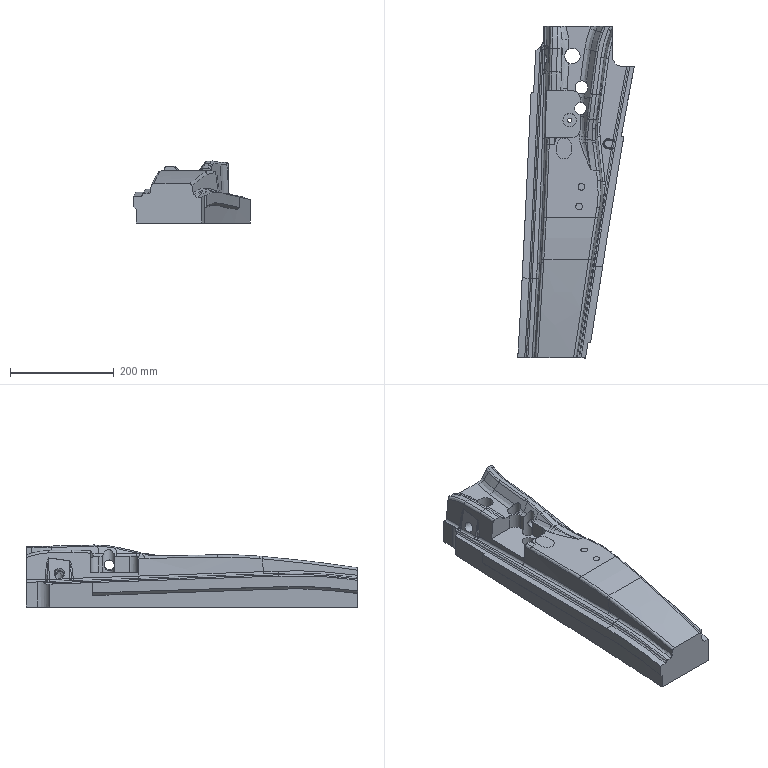Part | NX | features solid 2 | 1 solid | 192 faces | box 224.665 x 640.001 x 119.771 mm | volume 7956177 mm3 | spline 157 | plane 19 | cylinder 16 | commonest cylinder face diameters 20 x4 25 x3 30 x3 8 x1 16 x1 23 x1